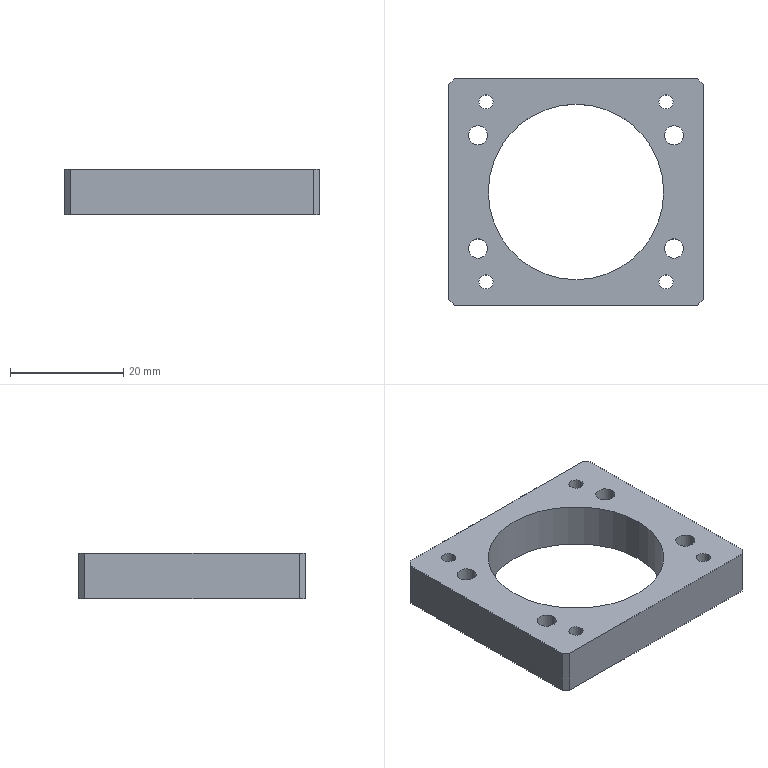Part | NX | features BREP 1 | 1 solid | 40 faces | box 45 x 40 x 8 mm | volume 7532 mm3 | cylinder 26 | plane 14 | commonest cylinder face diameters 2.5 x8 3.4 x8 6.7 x8 31 x2
STEP:
#1=CARTESIAN_POINT('',(-14.66,15.91,8.));
#2=VERTEX_POINT('',#1);
#3=CARTESIAN_POINT('',(-17.16,15.91,8.));
#4=VERTEX_POINT('',#3);
#5=CARTESIAN_POINT('',(-15.91,15.91,8.));
#6=DIRECTION('',(0.,0.,-1.));
#7=DIRECTION('',(-1.,0.,0.));
#8=AXIS2_PLACEMENT_3D('',#5,#6,#7);
#9=CIRCLE('',#8,1.25);
#10=EDGE_CURVE('',#2,#4,#9,.T.);
#11=ORIENTED_EDGE('',*,*,#10,.F.);
#12=CARTESIAN_POINT('',(-14.66,15.91,0.));
#13=VERTEX_POINT('',#12);
#14=CARTESIAN_POINT('',(-14.66,15.91,0.));
#15=DIRECTION('',(0.,0.,-1.));
#16=VECTOR('',#15,1000.);
#17=LINE('',#14,#16);
#18=EDGE_CURVE('',#2,#13,#17,.T.);
#19=ORIENTED_EDGE('',*,*,#18,.T.);
#20=CARTESIAN_POINT('',(-17.16,15.91,0.));
#21=VERTEX_POINT('',#20);
#22=CARTESIAN_POINT('',(-15.91,15.91,0.));
#23=DIRECTION('',(0.,0.,-1.));
#24=DIRECTION('',(-1.,0.,0.));
#25=AXIS2_PLACEMENT_3D('',#22,#23,#24);
#26=CIRCLE('',#25,1.25);
#27=EDGE_CURVE('',#13,#21,#26,.T.);
#28=ORIENTED_EDGE('',*,*,#27,.T.);
#29=CARTESIAN_POINT('',(-17.16,15.91,0.));
#30=DIRECTION('',(0.,0.,-1.));
#31=VECTOR('',#30,1000.);
#32=LINE('',#29,#31);
#33=EDGE_CURVE('',#4,#21,#32,.T.);
#34=ORIENTED_EDGE('',*,*,#33,.F.);
#35=EDGE_LOOP('',(#11,#19,#28,#34));
#36=FACE_BOUND('',#35,.T.);
#37=CARTESIAN_POINT('',(-15.91,15.91,0.));
#38=DIRECTION('',(0.,0.,-1.));
#39=DIRECTION('',(-1.,0.,0.));
#40=AXIS2_PLACEMENT_3D('',#37,#38,#39);
#41=CYLINDRICAL_SURFACE('',#40,1.25);
#42=ADVANCED_FACE('',(#36),#41,.F.);
#43=CARTESIAN_POINT('',(17.16,15.91,8.));
#44=VERTEX_POINT('',#43);
#45=CARTESIAN_POINT('',(14.66,15.91,8.));
#46=VERTEX_POINT('',#45);
#47=CARTESIAN_POINT('',(15.91,15.91,8.));
#48=DIRECTION('',(0.,0.,-1.));
#49=DIRECTION('',(-1.,0.,0.));
#50=AXIS2_PLACEMENT_3D('',#47,#48,#49);
#51=CIRCLE('',#50,1.25);
#52=EDGE_CURVE('',#44,#46,#51,.T.);
#53=ORIENTED_EDGE('',*,*,#52,.F.);
#54=CARTESIAN_POINT('',(17.16,15.91,0.));
#55=VERTEX_POINT('',#54);
#56=CARTESIAN_POINT('',(17.16,15.91,0.));
#57=DIRECTION('',(0.,0.,-1.));
#58=VECTOR('',#57,1000.);
#59=LINE('',#56,#58);
#60=EDGE_CURVE('',#44,#55,#59,.T.);
#61=ORIENTED_EDGE('',*,*,#60,.T.);
#62=CARTESIAN_POINT('',(14.66,15.91,0.));
#63=VERTEX_POINT('',#62);
#64=CARTESIAN_POINT('',(15.91,15.91,0.));
#65=DIRECTION('',(0.,0.,-1.));
#66=DIRECTION('',(-1.,0.,0.));
#67=AXIS2_PLACEMENT_3D('',#64,#65,#66);
#68=CIRCLE('',#67,1.25);
#69=EDGE_CURVE('',#55,#63,#68,.T.);
#70=ORIENTED_EDGE('',*,*,#69,.T.);
#71=CARTESIAN_POINT('',(14.66,15.91,0.));
#72=DIRECTION('',(0.,0.,-1.));
#73=VECTOR('',#72,1000.);
#74=LINE('',#71,#73);
#75=EDGE_CURVE('',#46,#63,#74,.T.);
#76=ORIENTED_EDGE('',*,*,#75,.F.);
#77=EDGE_LOOP('',(#53,#61,#70,#76));
#78=FACE_BOUND('',#77,.T.);
#79=CARTESIAN_POINT('',(15.91,15.91,0.));
#80=DIRECTION('',(0.,0.,-1.));
#81=DIRECTION('',(-1.,0.,0.));
#82=AXIS2_PLACEMENT_3D('',#79,#80,#81);
#83=CYLINDRICAL_SURFACE('',#82,1.25);
#84=ADVANCED_FACE('',(#78),#83,.F.);
#85=CARTESIAN_POINT('',(17.16,-15.91,8.));
#86=VERTEX_POINT('',#85);
#87=CARTESIAN_POINT('',(14.66,-15.91,8.));
#88=VERTEX_POINT('',#87);
#89=CARTESIAN_POINT('',(15.91,-15.91,8.));
#90=DIRECTION('',(0.,0.,-1.));
#91=DIRECTION('',(-1.,0.,0.));
#92=AXIS2_PLACEMENT_3D('',#89,#90,#91);
#93=CIRCLE('',#92,1.25);
#94=EDGE_CURVE('',#86,#88,#93,.T.);
#95=ORIENTED_EDGE('',*,*,#94,.F.);
#96=CARTESIAN_POINT('',(17.16,-15.91,0.));
#97=VERTEX_POINT('',#96);
#98=CARTESIAN_POINT('',(17.16,-15.91,0.));
#99=DIRECTION('',(0.,0.,-1.));
#100=VECTOR('',#99,1000.);
#101=LINE('',#98,#100);
#102=EDGE_CURVE('',#86,#97,#101,.T.);
#103=ORIENTED_EDGE('',*,*,#102,.T.);
#104=CARTESIAN_POINT('',(14.66,-15.91,0.));
#105=VERTEX_POINT('',#104);
#106=CARTESIAN_POINT('',(15.91,-15.91,0.));
#107=DIRECTION('',(0.,0.,-1.));
#108=DIRECTION('',(-1.,0.,0.));
#109=AXIS2_PLACEMENT_3D('',#106,#107,#108);
#110=CIRCLE('',#109,1.25);
#111=EDGE_CURVE('',#97,#105,#110,.T.);
#112=ORIENTED_EDGE('',*,*,#111,.T.);
#113=CARTESIAN_POINT('',(14.66,-15.91,0.));
#114=DIRECTION('',(0.,0.,-1.));
#115=VECTOR('',#114,1000.);
#116=LINE('',#113,#115);
#117=EDGE_CURVE('',#88,#105,#116,.T.);
#118=ORIENTED_EDGE('',*,*,#117,.F.);
#119=EDGE_LOOP('',(#95,#103,#112,#118));
#120=FACE_BOUND('',#119,.T.);
#121=CARTESIAN_POINT('',(15.91,-15.91,0.));
#122=DIRECTION('',(0.,0.,-1.));
#123=DIRECTION('',(-1.,0.,0.));
#124=AXIS2_PLACEMENT_3D('',#121,#122,#123);
#125=CYLINDRICAL_SURFACE('',#124,1.25);
#126=ADVANCED_FACE('',(#120),#125,.F.);
#127=CARTESIAN_POINT('',(-14.66,-15.91,8.));
#128=VERTEX_POINT('',#127);
#129=CARTESIAN_POINT('',(-17.16,-15.91,8.));
#130=VERTEX_POINT('',#129);
#131=CARTESIAN_POINT('',(-15.91,-15.91,8.));
#132=DIRECTION('',(0.,0.,-1.));
#133=DIRECTION('',(-1.,0.,0.));
#134=AXIS2_PLACEMENT_3D('',#131,#132,#133);
#135=CIRCLE('',#134,1.25);
#136=EDGE_CURVE('',#128,#130,#135,.T.);
#137=ORIENTED_EDGE('',*,*,#136,.F.);
#138=CARTESIAN_POINT('',(-14.66,-15.91,0.));
#139=VERTEX_POINT('',#138);
#140=CARTESIAN_POINT('',(-14.66,-15.91,0.));
#141=DIRECTION('',(0.,0.,-1.));
#142=VECTOR('',#141,1000.);
#143=LINE('',#140,#142);
#144=EDGE_CURVE('',#128,#139,#143,.T.);
#145=ORIENTED_EDGE('',*,*,#144,.T.);
#146=CARTESIAN_POINT('',(-17.16,-15.91,0.));
#147=VERTEX_POINT('',#146);
#148=CARTESIAN_POINT('',(-15.91,-15.91,0.));
#149=DIRECTION('',(0.,0.,-1.));
#150=DIRECTION('',(-1.,0.,0.));
#151=AXIS2_PLACEMENT_3D('',#148,#149,#150);
#152=CIRCLE('',#151,1.25);
#153=EDGE_CURVE('',#139,#147,#152,.T.);
#154=ORIENTED_EDGE('',*,*,#153,.T.);
#155=CARTESIAN_POINT('',(-17.16,-15.91,0.));
#156=DIRECTION('',(0.,0.,-1.));
#157=VECTOR('',#156,1000.);
#158=LINE('',#155,#157);
#159=EDGE_CURVE('',#130,#147,#158,.T.);
#160=ORIENTED_EDGE('',*,*,#159,.F.);
#161=EDGE_LOOP('',(#137,#145,#154,#160));
#162=FACE_BOUND('',#161,.T.);
#163=CARTESIAN_POINT('',(-15.91,-15.91,0.));
#164=DIRECTION('',(0.,0.,-1.));
#165=DIRECTION('',(-1.,0.,0.));
#166=AXIS2_PLACEMENT_3D('',#163,#164,#165);
#167=CYLINDRICAL_SURFACE('',#166,1.25);
#168=ADVANCED_FACE('',(#162),#167,.F.);
#169=CARTESIAN_POINT('',(-13.971,-10.,3.5));
#170=VERTEX_POINT('',#169);
#171=CARTESIAN_POINT('',(-20.671,-10.,3.5));
#172=VERTEX_POINT('',#171);
#173=CARTESIAN_POINT('',(-17.321,-10.,3.5));
#174=DIRECTION('',(0.,0.,-1.));
#175=DIRECTION('',(-1.,0.,0.));
#176=AXIS2_PLACEMENT_3D('',#173,#174,#175);
#177=CIRCLE('',#176,3.35);
#178=EDGE_CURVE('',#170,#172,#177,.T.);
#179=ORIENTED_EDGE('',*,*,#178,.F.);
#180=CARTESIAN_POINT('',(-13.971,-10.,0.));
#181=VERTEX_POINT('',#180);
#182=CARTESIAN_POINT('',(-13.971,-10.,0.));
#183=DIRECTION('',(0.,0.,-1.));
#184=VECTOR('',#183,1000.);
#185=LINE('',#182,#184);
#186=EDGE_CURVE('',#170,#181,#185,.T.);
#187=ORIENTED_EDGE('',*,*,#186,.T.);
#188=CARTESIAN_POINT('',(-20.671,-10.,0.));
#189=VERTEX_POINT('',#188);
#190=CARTESIAN_POINT('',(-17.321,-10.,0.));
#191=DIRECTION('',(0.,0.,-1.));
#192=DIRECTION('',(-1.,0.,0.));
#193=AXIS2_PLACEMENT_3D('',#190,#191,#192);
#194=CIRCLE('',#193,3.35);
#195=EDGE_CURVE('',#181,#189,#194,.T.);
#196=ORIENTED_EDGE('',*,*,#195,.T.);
#197=CARTESIAN_POINT('',(-20.671,-10.,0.));
#198=DIRECTION('',(0.,0.,-1.));
#199=VECTOR('',#198,1000.);
#200=LINE('',#197,#199);
#201=EDGE_CURVE('',#172,#189,#200,.T.);
#202=ORIENTED_EDGE('',*,*,#201,.F.);
#203=EDGE_LOOP('',(#179,#187,#196,#202));
#204=FACE_BOUND('',#203,.T.);
#205=CARTESIAN_POINT('',(-17.321,-10.,0.));
#206=DIRECTION('',(0.,0.,-1.));
#207=DIRECTION('',(-1.,0.,0.));
#208=AXIS2_PLACEMENT_3D('',#205,#206,#207);
#209=CYLINDRICAL_SURFACE('',#208,3.35);
#210=ADVANCED_FACE('',(#204),#209,.F.);
#211=CARTESIAN_POINT('',(-15.621,-10.,8.));
#212=VERTEX_POINT('',#211);
#213=CARTESIAN_POINT('',(-19.021,-10.,8.));
#214=VERTEX_POINT('',#213);
#215=CARTESIAN_POINT('',(-17.321,-10.,8.));
#216=DIRECTION('',(0.,0.,-1.));
#217=DIRECTION('',(-1.,0.,0.));
#218=AXIS2_PLACEMENT_3D('',#215,#216,#217);
#219=CIRCLE('',#218,1.7);
#220=EDGE_CURVE('',#212,#214,#219,.T.);
#221=ORIENTED_EDGE('',*,*,#220,.F.);
#222=CARTESIAN_POINT('',(-15.621,-10.,3.5));
#223=VERTEX_POINT('',#222);
#224=CARTESIAN_POINT('',(-15.621,-10.,0.));
#225=DIRECTION('',(0.,0.,-1.));
#226=VECTOR('',#225,1000.);
#227=LINE('',#224,#226);
#228=EDGE_CURVE('',#212,#223,#227,.T.);
#229=ORIENTED_EDGE('',*,*,#228,.T.);
#230=CARTESIAN_POINT('',(-19.021,-10.,3.5));
#231=VERTEX_POINT('',#230);
#232=CARTESIAN_POINT('',(-17.321,-10.,3.5));
#233=DIRECTION('',(0.,0.,-1.));
#234=DIRECTION('',(-1.,0.,0.));
#235=AXIS2_PLACEMENT_3D('',#232,#233,#234);
#236=CIRCLE('',#235,1.7);
#237=EDGE_CURVE('',#223,#231,#236,.T.);
#238=ORIENTED_EDGE('',*,*,#237,.T.);
#239=CARTESIAN_POINT('',(-19.021,-10.,0.));
#240=DIRECTION('',(0.,0.,-1.));
#241=VECTOR('',#240,1000.);
#242=LINE('',#239,#241);
#243=EDGE_CURVE('',#214,#231,#242,.T.);
#244=ORIENTED_EDGE('',*,*,#243,.F.);
#245=EDGE_LOOP('',(#221,#229,#238,#244));
#246=FACE_BOUND('',#245,.T.);
#247=CARTESIAN_POINT('',(-17.321,-10.,0.));
#248=DIRECTION('',(0.,0.,-1.));
#249=DIRECTION('',(-1.,0.,0.));
#250=AXIS2_PLACEMENT_3D('',#247,#248,#249);
#251=CYLINDRICAL_SURFACE('',#250,1.7);
#252=ADVANCED_FACE('',(#246),#251,.F.);
#253=CARTESIAN_POINT('',(-13.971,10.,3.5));
#254=VERTEX_POINT('',#253);
#255=CARTESIAN_POINT('',(-20.671,10.,3.5));
#256=VERTEX_POINT('',#255);
#257=CARTESIAN_POINT('',(-17.321,10.,3.5));
#258=DIRECTION('',(0.,0.,-1.));
#259=DIRECTION('',(-1.,0.,0.));
#260=AXIS2_PLACEMENT_3D('',#257,#258,#259);
#261=CIRCLE('',#260,3.35);
#262=EDGE_CURVE('',#254,#256,#261,.T.);
#263=ORIENTED_EDGE('',*,*,#262,.F.);
#264=CARTESIAN_POINT('',(-13.971,10.,0.));
#265=VERTEX_POINT('',#264);
#266=CARTESIAN_POINT('',(-13.971,10.,0.));
#267=DIRECTION('',(0.,0.,-1.));
#268=VECTOR('',#267,1000.);
#269=LINE('',#266,#268);
#270=EDGE_CURVE('',#254,#265,#269,.T.);
#271=ORIENTED_EDGE('',*,*,#270,.T.);
#272=CARTESIAN_POINT('',(-20.671,10.,0.));
#273=VERTEX_POINT('',#272);
#274=CARTESIAN_POINT('',(-17.321,10.,0.));
#275=DIRECTION('',(0.,0.,-1.));
#276=DIRECTION('',(-1.,0.,0.));
#277=AXIS2_PLACEMENT_3D('',#274,#275,#276);
#278=CIRCLE('',#277,3.35);
#279=EDGE_CURVE('',#265,#273,#278,.T.);
#280=ORIENTED_EDGE('',*,*,#279,.T.);
#281=CARTESIAN_POINT('',(-20.671,10.,0.));
#282=DIRECTION('',(0.,0.,-1.));
#283=VECTOR('',#282,1000.);
#284=LINE('',#281,#283);
#285=EDGE_CURVE('',#256,#273,#284,.T.);
#286=ORIENTED_EDGE('',*,*,#285,.F.);
#287=EDGE_LOOP('',(#263,#271,#280,#286));
#288=FACE_BOUND('',#287,.T.);
#289=CARTESIAN_POINT('',(-17.321,10.,0.));
#290=DIRECTION('',(0.,0.,-1.));
#291=DIRECTION('',(-1.,0.,0.));
#292=AXIS2_PLACEMENT_3D('',#289,#290,#291);
#293=CYLINDRICAL_SURFACE('',#292,3.35);
#294=ADVANCED_FACE('',(#288),#293,.F.);
#295=CARTESIAN_POINT('',(-15.621,10.,8.));
#296=VERTEX_POINT('',#295);
#297=CARTESIAN_POINT('',(-19.021,10.,8.));
#298=VERTEX_POINT('',#297);
#299=CARTESIAN_POINT('',(-17.321,10.,8.));
#300=DIRECTION('',(0.,0.,-1.));
#301=DIRECTION('',(-1.,0.,0.));
#302=AXIS2_PLACEMENT_3D('',#299,#300,#301);
#303=CIRCLE('',#302,1.7);
#304=EDGE_CURVE('',#296,#298,#303,.T.);
#305=ORIENTED_EDGE('',*,*,#304,.F.);
#306=CARTESIAN_POINT('',(-15.621,10.,3.5));
#307=VERTEX_POINT('',#306);
#308=CARTESIAN_POINT('',(-15.621,10.,0.));
#309=DIRECTION('',(0.,0.,-1.));
#310=VECTOR('',#309,1000.);
#311=LINE('',#308,#310);
#312=EDGE_CURVE('',#296,#307,#311,.T.);
#313=ORIENTED_EDGE('',*,*,#312,.T.);
#314=CARTESIAN_POINT('',(-19.021,10.,3.5));
#315=VERTEX_POINT('',#314);
#316=CARTESIAN_POINT('',(-17.321,10.,3.5));
#317=DIRECTION('',(0.,0.,-1.));
#318=DIRECTION('',(-1.,0.,0.));
#319=AXIS2_PLACEMENT_3D('',#316,#317,#318);
#320=CIRCLE('',#319,1.7);
#321=EDGE_CURVE('',#307,#315,#320,.T.);
#322=ORIENTED_EDGE('',*,*,#321,.T.);
#323=CARTESIAN_POINT('',(-19.021,10.,0.));
#324=DIRECTION('',(0.,0.,-1.));
#325=VECTOR('',#324,1000.);
#326=LINE('',#323,#325);
#327=EDGE_CURVE('',#298,#315,#326,.T.);
#328=ORIENTED_EDGE('',*,*,#327,.F.);
#329=EDGE_LOOP('',(#305,#313,#322,#328));
#330=FACE_BOUND('',#329,.T.);
#331=CARTESIAN_POINT('',(-17.321,10.,0.));
#332=DIRECTION('',(0.,0.,-1.));
#333=DIRECTION('',(-1.,0.,0.));
#334=AXIS2_PLACEMENT_3D('',#331,#332,#333);
#335=CYLINDRICAL_SURFACE('',#334,1.7);
#336=ADVANCED_FACE('',(#330),#335,.F.);
#337=CARTESIAN_POINT('',(20.671,10.,3.5));
#338=VERTEX_POINT('',#337);
#339=CARTESIAN_POINT('',(13.971,10.,3.5));
#340=VERTEX_POINT('',#339);
#341=CARTESIAN_POINT('',(17.321,10.,3.5));
#342=DIRECTION('',(0.,0.,-1.));
#343=DIRECTION('',(-1.,0.,0.));
#344=AXIS2_PLACEMENT_3D('',#341,#342,#343);
#345=CIRCLE('',#344,3.35);
#346=EDGE_CURVE('',#338,#340,#345,.T.);
#347=ORIENTED_EDGE('',*,*,#346,.F.);
#348=CARTESIAN_POINT('',(20.671,10.,0.));
#349=VERTEX_POINT('',#348);
#350=CARTESIAN_POINT('',(20.671,10.,0.));
#351=DIRECTION('',(0.,0.,-1.));
#352=VECTOR('',#351,1000.);
#353=LINE('',#350,#352);
#354=EDGE_CURVE('',#338,#349,#353,.T.);
#355=ORIENTED_EDGE('',*,*,#354,.T.);
#356=CARTESIAN_POINT('',(13.971,10.,0.));
#357=VERTEX_POINT('',#356);
#358=CARTESIAN_POINT('',(17.321,10.,0.));
#359=DIRECTION('',(0.,0.,-1.));
#360=DIRECTION('',(-1.,0.,0.));
#361=AXIS2_PLACEMENT_3D('',#358,#359,#360);
#362=CIRCLE('',#361,3.35);
#363=EDGE_CURVE('',#349,#357,#362,.T.);
#364=ORIENTED_EDGE('',*,*,#363,.T.);
#365=CARTESIAN_POINT('',(13.971,10.,0.));
#366=DIRECTION('',(0.,0.,-1.));
#367=VECTOR('',#366,1000.);
#368=LINE('',#365,#367);
#369=EDGE_CURVE('',#340,#357,#368,.T.);
#370=ORIENTED_EDGE('',*,*,#369,.F.);
#371=EDGE_LOOP('',(#347,#355,#364,#370));
#372=FACE_BOUND('',#371,.T.);
#373=CARTESIAN_POINT('',(17.321,10.,0.));
#374=DIRECTION('',(0.,0.,-1.));
#375=DIRECTION('',(-1.,0.,0.));
#376=AXIS2_PLACEMENT_3D('',#373,#374,#375);
#377=CYLINDRICAL_SURFACE('',#376,3.35);
#378=ADVANCED_FACE('',(#372),#377,.F.);
#379=CARTESIAN_POINT('',(19.021,10.,8.));
#380=VERTEX_POINT('',#379);
#381=CARTESIAN_POINT('',(15.621,10.,8.));
#382=VERTEX_POINT('',#381);
#383=CARTESIAN_POINT('',(17.321,10.,8.));
#384=DIRECTION('',(0.,0.,-1.));
#385=DIRECTION('',(-1.,0.,0.));
#386=AXIS2_PLACEMENT_3D('',#383,#384,#385);
#387=CIRCLE('',#386,1.7);
#388=EDGE_CURVE('',#380,#382,#387,.T.);
#389=ORIENTED_EDGE('',*,*,#388,.F.);
#390=CARTESIAN_POINT('',(19.021,10.,3.5));
#391=VERTEX_POINT('',#390);
#392=CARTESIAN_POINT('',(19.021,10.,0.));
#393=DIRECTION('',(0.,0.,-1.));
#394=VECTOR('',#393,1000.);
#395=LINE('',#392,#394);
#396=EDGE_CURVE('',#380,#391,#395,.T.);
#397=ORIENTED_EDGE('',*,*,#396,.T.);
#398=CARTESIAN_POINT('',(15.621,10.,3.5));
#399=VERTEX_POINT('',#398);
#400=CARTESIAN_POINT('',(17.321,10.,3.5));
#401=DIRECTION('',(0.,0.,-1.));
#402=DIRECTION('',(-1.,0.,0.));
#403=AXIS2_PLACEMENT_3D('',#400,#401,#402);
#404=CIRCLE('',#403,1.7);
#405=EDGE_CURVE('',#391,#399,#404,.T.);
#406=ORIENTED_EDGE('',*,*,#405,.T.);
#407=CARTESIAN_POINT('',(15.621,10.,0.));
#408=DIRECTION('',(0.,0.,-1.));
#409=VECTOR('',#408,1000.);
#410=LINE('',#407,#409);
#411=EDGE_CURVE('',#382,#399,#410,.T.);
#412=ORIENTED_EDGE('',*,*,#411,.F.);
#413=EDGE_LOOP('',(#389,#397,#406,#412));
#414=FACE_BOUND('',#413,.T.);
#415=CARTESIAN_POINT('',(17.321,10.,0.));
#416=DIRECTION('',(0.,0.,-1.));
#417=DIRECTION('',(-1.,0.,0.));
#418=AXIS2_PLACEMENT_3D('',#415,#416,#417);
#419=CYLINDRICAL_SURFACE('',#418,1.7);
#420=ADVANCED_FACE('',(#414),#419,.F.);
#421=CARTESIAN_POINT('',(20.671,-10.,3.5));
#422=VERTEX_POINT('',#421);
#423=CARTESIAN_POINT('',(13.971,-10.,3.5));
#424=VERTEX_POINT('',#423);
#425=CARTESIAN_POINT('',(17.321,-10.,3.5));
#426=DIRECTION('',(0.,0.,-1.));
#427=DIRECTION('',(-1.,0.,0.));
#428=AXIS2_PLACEMENT_3D('',#425,#426,#427);
#429=CIRCLE('',#428,3.35);
#430=EDGE_CURVE('',#422,#424,#429,.T.);
#431=ORIENTED_EDGE('',*,*,#430,.F.);
#432=CARTESIAN_POINT('',(20.671,-10.,0.));
#433=VERTEX_POINT('',#432);
#434=CARTESIAN_POINT('',(20.671,-10.,0.));
#435=DIRECTION('',(0.,0.,-1.));
#436=VECTOR('',#435,1000.);
#437=LINE('',#434,#436);
#438=EDGE_CURVE('',#422,#433,#437,.T.);
#439=ORIENTED_EDGE('',*,*,#438,.T.);
#440=CARTESIAN_POINT('',(13.971,-10.,0.));
#441=VERTEX_POINT('',#440);
#442=CARTESIAN_POINT('',(17.321,-10.,0.));
#443=DIRECTION('',(0.,0.,-1.));
#444=DIRECTION('',(-1.,0.,0.));
#445=AXIS2_PLACEMENT_3D('',#442,#443,#444);
#446=CIRCLE('',#445,3.35);
#447=EDGE_CURVE('',#433,#441,#446,.T.);
#448=ORIENTED_EDGE('',*,*,#447,.T.);
#449=CARTESIAN_POINT('',(13.971,-10.,0.));
#450=DIRECTION('',(0.,0.,-1.));
#451=VECTOR('',#450,1000.);
#452=LINE('',#449,#451);
#453=EDGE_CURVE('',#424,#441,#452,.T.);
#454=ORIENTED_EDGE('',*,*,#453,.F.);
#455=EDGE_LOOP('',(#431,#439,#448,#454));
#456=FACE_BOUND('',#455,.T.);
#457=CARTESIAN_POINT('',(17.321,-10.,0.));
#458=DIRECTION('',(0.,0.,-1.));
#459=DIRECTION('',(-1.,0.,0.));
#460=AXIS2_PLACEMENT_3D('',#457,#458,#459);
#461=CYLINDRICAL_SURFACE('',#460,3.35);
#462=ADVANCED_FACE('',(#456),#461,.F.);
#463=CARTESIAN_POINT('',(19.021,-10.,8.));
#464=VERTEX_POINT('',#463);
#465=CARTESIAN_POINT('',(15.621,-10.,8.));
#466=VERTEX_POINT('',#465);
#467=CARTESIAN_POINT('',(17.321,-10.,8.));
#468=DIRECTION('',(0.,0.,-1.));
#469=DIRECTION('',(-1.,0.,0.));
#470=AXIS2_PLACEMENT_3D('',#467,#468,#469);
#471=CIRCLE('',#470,1.7);
#472=EDGE_CURVE('',#464,#466,#471,.T.);
#473=ORIENTED_EDGE('',*,*,#472,.F.);
#474=CARTESIAN_POINT('',(19.021,-10.,3.5));
#475=VERTEX_POINT('',#474);
#476=CARTESIAN_POINT('',(19.021,-10.,0.));
#477=DIRECTION('',(0.,0.,-1.));
#478=VECTOR('',#477,1000.);
#479=LINE('',#476,#478);
#480=EDGE_CURVE('',#464,#475,#479,.T.);
#481=ORIENTED_EDGE('',*,*,#480,.T.);
#482=CARTESIAN_POINT('',(15.621,-10.,3.5));
#483=VERTEX_POINT('',#482);
#484=CARTESIAN_POINT('',(17.321,-10.,3.5));
#485=DIRECTION('',(0.,0.,-1.));
#486=DIRECTION('',(-1.,0.,0.));
#487=AXIS2_PLACEMENT_3D('',#484,#485,#486);
#488=CIRCLE('',#487,1.7);
#489=EDGE_CURVE('',#475,#483,#488,.T.);
#490=ORIENTED_EDGE('',*,*,#489,.T.);
#491=CARTESIAN_POINT('',(15.621,-10.,0.));
#492=DIRECTION('',(0.,0.,-1.));
#493=VECTOR('',#492,1000.);
#494=LINE('',#491,#493);
#495=EDGE_CURVE('',#466,#483,#494,.T.);
#496=ORIENTED_EDGE('',*,*,#495,.F.);
#497=EDGE_LOOP('',(#473,#481,#490,#496));
#498=FACE_BOUND('',#497,.T.);
#499=CARTESIAN_POINT('',(17.321,-10.,0.));
#500=DIRECTION('',(0.,0.,-1.));
#501=DIRECTION('',(-1.,0.,0.));
#502=AXIS2_PLACEMENT_3D('',#499,#500,#501);
#503=CYLINDRICAL_SURFACE('',#502,1.7);
#504=ADVANCED_FACE('',(#498),#503,.F.);
#505=CARTESIAN_POINT('',(-15.5,0.,0.));
#506=VERTEX_POINT('',#505);
#507=CARTESIAN_POINT('',(15.5,0.,0.));
#508=VERTEX_POINT('',#507);
#509=CARTESIAN_POINT('',(0.,0.,0.));
#510=DIRECTION('',(0.,0.,1.));
#511=DIRECTION('',(1.,0.,0.));
#512=AXIS2_PLACEMENT_3D('',#509,#510,#511);
#513=CIRCLE('',#512,15.5);
#514=EDGE_CURVE('',#506,#508,#513,.T.);
#515=ORIENTED_EDGE('',*,*,#514,.F.);
#516=CARTESIAN_POINT('',(-15.5,0.,8.));
#517=VERTEX_POINT('',#516);
#518=CARTESIAN_POINT('',(-15.5,0.,-20.));
#519=DIRECTION('',(0.,0.,1.));
#520=VECTOR('',#519,1000.);
#521=LINE('',#518,#520);
#522=EDGE_CURVE('',#517,#506,#521,.F.);
#523=ORIENTED_EDGE('',*,*,#522,.F.);
#524=CARTESIAN_POINT('',(15.5,0.,8.));
#525=VERTEX_POINT('',#524);
#526=CARTESIAN_POINT('',(0.,0.,8.));
#527=DIRECTION('',(0.,0.,1.));
#528=DIRECTION('',(1.,0.,0.));
#529=AXIS2_PLACEMENT_3D('',#526,#527,#528);
#530=CIRCLE('',#529,15.5);
#531=EDGE_CURVE('',#517,#525,#530,.T.);
#532=ORIENTED_EDGE('',*,*,#531,.T.);
#533=CARTESIAN_POINT('',(15.5,0.,-20.));
#534=DIRECTION('',(0.,0.,1.));
#535=VECTOR('',#534,1000.);
#536=LINE('',#533,#535);
#537=EDGE_CURVE('',#525,#508,#536,.F.);
#538=ORIENTED_EDGE('',*,*,#537,.T.);
#539=EDGE_LOOP('',(#515,#523,#532,#538));
#540=FACE_BOUND('',#539,.T.);
#541=CARTESIAN_POINT('',(0.,0.,-20.));
#542=DIRECTION('',(0.,0.,1.));
#543=DIRECTION('',(1.,0.,0.));
#544=AXIS2_PLACEMENT_3D('',#541,#542,#543);
#545=CYLINDRICAL_SURFACE('',#544,15.5);
#546=ADVANCED_FACE('',(#540),#545,.F.);
#547=CARTESIAN_POINT('',(22.5,-19.,8.));
#548=VERTEX_POINT('',#547);
#549=CARTESIAN_POINT('',(22.5,19.,8.));
#550=VERTEX_POINT('',#549);
#551=CARTESIAN_POINT('',(22.5,20.,8.));
#552=DIRECTION('',(0.,1.,0.));
#553=VECTOR('',#552,1000.);
#554=LINE('',#551,#553);
#555=EDGE_CURVE('',#548,#550,#554,.T.);
#556=ORIENTED_EDGE('',*,*,#555,.F.);
#557=CARTESIAN_POINT('',(22.5,-19.,0.));
#558=VERTEX_POINT('',#557);
#559=CARTESIAN_POINT('',(22.5,-19.,8.));
#560=DIRECTION('',(0.,0.,-1.));
#561=VECTOR('',#560,1000.);
#562=LINE('',#559,#561);
#563=EDGE_CURVE('',#548,#558,#562,.T.);
#564=ORIENTED_EDGE('',*,*,#563,.T.);
#565=CARTESIAN_POINT('',(22.5,19.,0.));
#566=VERTEX_POINT('',#565);
#567=CARTESIAN_POINT('',(22.5,20.,0.));
#568=DIRECTION('',(0.,1.,0.));
#569=VECTOR('',#568,1000.);
#570=LINE('',#567,#569);
#571=EDGE_CURVE('',#558,#566,#570,.T.);
#572=ORIENTED_EDGE('',*,*,#571,.T.);
#573=CARTESIAN_POINT('',(22.5,19.,8.));
#574=DIRECTION('',(0.,0.,1.));
#575=VECTOR('',#574,1000.);
#576=LINE('',#573,#575);
#577=EDGE_CURVE('',#566,#550,#576,.T.);
#578=ORIENTED_EDGE('',*,*,#577,.T.);
#579=EDGE_LOOP('',(#556,#564,#572,#578));
#580=FACE_BOUND('',#579,.T.);
#581=CARTESIAN_POINT('',(22.5,20.,8.));
#582=DIRECTION('',(-1.,0.,0.));
#583=DIRECTION('',(0.,1.,0.));
#584=AXIS2_PLACEMENT_3D('',#581,#582,#583);
#585=PLANE('',#584);
#586=ADVANCED_FACE('',(#580),#585,.F.);
#587=CARTESIAN_POINT('',(21.5,20.,8.));
#588=VERTEX_POINT('',#587);
#589=CARTESIAN_POINT('',(-21.5,20.,8.));
#590=VERTEX_POINT('',#589);
#591=CARTESIAN_POINT('',(-22.5,20.,8.));
#592=DIRECTION('',(-1.,0.,0.));
#593=VECTOR('',#592,1000.);
#594=LINE('',#591,#593);
#595=EDGE_CURVE('',#588,#590,#594,.T.);
#596=ORIENTED_EDGE('',*,*,#595,.F.);
#597=CARTESIAN_POINT('',(21.5,20.,0.));
#598=VERTEX_POINT('',#597);
#599=CARTESIAN_POINT('',(21.5,20.,8.));
#600=DIRECTION('',(0.,0.,-1.));
#601=VECTOR('',#600,1000.);
#602=LINE('',#599,#601);
#603=EDGE_CURVE('',#588,#598,#602,.T.);
#604=ORIENTED_EDGE('',*,*,#603,.T.);
#605=CARTESIAN_POINT('',(-21.5,20.,0.));
#606=VERTEX_POINT('',#605);
#607=CARTESIAN_POINT('',(-22.5,20.,0.));
#608=DIRECTION('',(-1.,0.,0.));
#609=VECTOR('',#608,1000.);
#610=LINE('',#607,#609);
#611=EDGE_CURVE('',#598,#606,#610,.T.);
#612=ORIENTED_EDGE('',*,*,#611,.T.);
#613=CARTESIAN_POINT('',(-21.5,20.,8.));
#614=DIRECTION('',(0.,0.,1.));
#615=VECTOR('',#614,1000.);
#616=LINE('',#613,#615);
#617=EDGE_CURVE('',#606,#590,#616,.T.);
#618=ORIENTED_EDGE('',*,*,#617,.T.);
#619=EDGE_LOOP('',(#596,#604,#612,#618));
#620=FACE_BOUND('',#619,.T.);
#621=CARTESIAN_POINT('',(-22.5,20.,8.));
#622=DIRECTION('',(0.,-1.,0.));
#623=DIRECTION('',(0.,0.,-1.));
#624=AXIS2_PLACEMENT_3D('',#621,#622,#623);
#625=PLANE('',#624);
#626=ADVANCED_FACE('',(#620),#625,.F.);
#627=CARTESIAN_POINT('',(-22.5,19.,0.));
#628=VERTEX_POINT('',#627);
#629=CARTESIAN_POINT('',(-22.5,-19.,0.));
#630=VERTEX_POINT('',#629);
#631=CARTESIAN_POINT('',(-22.5,20.,0.));
#632=DIRECTION('',(0.,-1.,0.));
#633=VECTOR('',#632,1000.);
#634=LINE('',#631,#633);
#635=EDGE_CURVE('',#628,#630,#634,.T.);
#636=ORIENTED_EDGE('',*,*,#635,.T.);
#637=CARTESIAN_POINT('',(-22.5,-19.,8.));
#638=VERTEX_POINT('',#637);
#639=CARTESIAN_POINT('',(-22.5,-19.,8.));
#640=DIRECTION('',(0.,0.,1.));
#641=VECTOR('',#640,1000.);
#642=LINE('',#639,#641);
#643=EDGE_CURVE('',#630,#638,#642,.T.);
#644=ORIENTED_EDGE('',*,*,#643,.T.);
#645=CARTESIAN_POINT('',(-22.5,19.,8.));
#646=VERTEX_POINT('',#645);
#647=CARTESIAN_POINT('',(-22.5,20.,8.));
#648=DIRECTION('',(0.,-1.,0.));
#649=VECTOR('',#648,1000.);
#650=LINE('',#647,#649);
#651=EDGE_CURVE('',#646,#638,#650,.T.);
#652=ORIENTED_EDGE('',*,*,#651,.F.);
#653=CARTESIAN_POINT('',(-22.5,19.,8.));
#654=DIRECTION('',(0.,0.,-1.));
#655=VECTOR('',#654,1000.);
#656=LINE('',#653,#655);
#657=EDGE_CURVE('',#646,#628,#656,.T.);
#658=ORIENTED_EDGE('',*,*,#657,.T.);
#659=EDGE_LOOP('',(#636,#644,#652,#658));
#660=FACE_BOUND('',#659,.T.);
#661=CARTESIAN_POINT('',(-22.5,20.,8.));
#662=DIRECTION('',(1.,0.,0.));
#663=DIRECTION('',(0.,1.,0.));
#664=AXIS2_PLACEMENT_3D('',#661,#662,#663);
#665=PLANE('',#664);
#666=ADVANCED_FACE('',(#660),#665,.F.);
#667=CARTESIAN_POINT('',(-21.5,-20.,8.));
#668=VERTEX_POINT('',#667);
#669=CARTESIAN_POINT('',(21.5,-20.,8.));
#670=VERTEX_POINT('',#669);
#671=CARTESIAN_POINT('',(-22.5,-20.,8.));
#672=DIRECTION('',(1.,0.,0.));
#673=VECTOR('',#672,1000.);
#674=LINE('',#671,#673);
#675=EDGE_CURVE('',#668,#670,#674,.T.);
#676=ORIENTED_EDGE('',*,*,#675,.F.);
#677=CARTESIAN_POINT('',(-21.5,-20.,0.));
#678=VERTEX_POINT('',#677);
#679=CARTESIAN_POINT('',(-21.5,-20.,8.));
#680=DIRECTION('',(0.,0.,-1.));
#681=VECTOR('',#680,1000.);
#682=LINE('',#679,#681);
#683=EDGE_CURVE('',#668,#678,#682,.T.);
#684=ORIENTED_EDGE('',*,*,#683,.T.);
#685=CARTESIAN_POINT('',(21.5,-20.,0.));
#686=VERTEX_POINT('',#685);
#687=CARTESIAN_POINT('',(-22.5,-20.,0.));
#688=DIRECTION('',(1.,0.,0.));
#689=VECTOR('',#688,1000.);
#690=LINE('',#687,#689);
#691=EDGE_CURVE('',#678,#686,#690,.T.);
#692=ORIENTED_EDGE('',*,*,#691,.T.);
#693=CARTESIAN_POINT('',(21.5,-20.,8.));
#694=DIRECTION('',(0.,0.,1.));
#695=VECTOR('',#694,1000.);
#696=LINE('',#693,#695);
#697=EDGE_CURVE('',#686,#670,#696,.T.);
#698=ORIENTED_EDGE('',*,*,#697,.T.);
#699=EDGE_LOOP('',(#676,#684,#692,#698));
#700=FACE_BOUND('',#699,.T.);
#701=CARTESIAN_POINT('',(-22.5,-20.,8.));
#702=DIRECTION('',(0.,1.,0.));
#703=DIRECTION('',(1.,0.,0.));
#704=AXIS2_PLACEMENT_3D('',#701,#702,#703);
#705=PLANE('',#704);
#706=ADVANCED_FACE('',(#700),#705,.F.);
#707=ORIENTED_EDGE('',*,*,#651,.T.);
#708=CARTESIAN_POINT('',(-20.75,-20.75,8.));
#709=DIRECTION('',(0.7071,-0.7071,0.));
#710=VECTOR('',#709,1000.);
#711=LINE('',#708,#710);
#712=EDGE_CURVE('',#638,#668,#711,.T.);
#713=ORIENTED_EDGE('',*,*,#712,.T.);
#714=ORIENTED_EDGE('',*,*,#675,.T.);
#715=CARTESIAN_POINT('',(20.75,-20.75,8.));
#716=DIRECTION('',(0.7071,0.7071,0.));
#717=VECTOR('',#716,1000.);
#718=LINE('',#715,#717);
#719=EDGE_CURVE('',#670,#548,#718,.T.);
#720=ORIENTED_EDGE('',*,*,#719,.T.);
#721=ORIENTED_EDGE('',*,*,#555,.T.);
#722=CARTESIAN_POINT('',(20.75,20.75,8.));
#723=DIRECTION('',(-0.7071,0.7071,0.));
#724=VECTOR('',#723,1000.);
#725=LINE('',#722,#724);
#726=EDGE_CURVE('',#550,#588,#725,.T.);
#727=ORIENTED_EDGE('',*,*,#726,.T.);
#728=ORIENTED_EDGE('',*,*,#595,.T.);
#729=CARTESIAN_POINT('',(-20.75,20.75,8.));
#730=DIRECTION('',(-0.7071,-0.7071,0.));
#731=VECTOR('',#730,1000.);
#732=LINE('',#729,#731);
#733=EDGE_CURVE('',#590,#646,#732,.T.);
#734=ORIENTED_EDGE('',*,*,#733,.T.);
#735=EDGE_LOOP('',(#707,#713,#714,#720,#721,#727,#728,#734));
#736=FACE_BOUND('',#735,.T.);
#737=CARTESIAN_POINT('',(-15.91,15.91,8.));
#738=DIRECTION('',(0.,0.,-1.));
#739=DIRECTION('',(-1.,0.,0.));
#740=AXIS2_PLACEMENT_3D('',#737,#738,#739);
#741=CIRCLE('',#740,1.25);
#742=EDGE_CURVE('',#4,#2,#741,.T.);
#743=ORIENTED_EDGE('',*,*,#742,.T.);
#744=ORIENTED_EDGE('',*,*,#10,.T.);
#745=EDGE_LOOP('',(#743,#744));
#746=FACE_BOUND('',#745,.T.);
#747=CARTESIAN_POINT('',(15.91,15.91,8.));
#748=DIRECTION('',(0.,0.,-1.));
#749=DIRECTION('',(-1.,0.,0.));
#750=AXIS2_PLACEMENT_3D('',#747,#748,#749);
#751=CIRCLE('',#750,1.25);
#752=EDGE_CURVE('',#46,#44,#751,.T.);
#753=ORIENTED_EDGE('',*,*,#752,.T.);
#754=ORIENTED_EDGE('',*,*,#52,.T.);
#755=EDGE_LOOP('',(#753,#754));
#756=FACE_BOUND('',#755,.T.);
#757=CARTESIAN_POINT('',(15.91,-15.91,8.));
#758=DIRECTION('',(0.,0.,-1.));
#759=DIRECTION('',(-1.,0.,0.));
#760=AXIS2_PLACEMENT_3D('',#757,#758,#759);
#761=CIRCLE('',#760,1.25);
#762=EDGE_CURVE('',#88,#86,#761,.T.);
#763=ORIENTED_EDGE('',*,*,#762,.T.);
#764=ORIENTED_EDGE('',*,*,#94,.T.);
#765=EDGE_LOOP('',(#763,#764));
#766=FACE_BOUND('',#765,.T.);
#767=CARTESIAN_POINT('',(-15.91,-15.91,8.));
#768=DIRECTION('',(0.,0.,-1.));
#769=DIRECTION('',(-1.,0.,0.));
#770=AXIS2_PLACEMENT_3D('',#767,#768,#769);
#771=CIRCLE('',#770,1.25);
#772=EDGE_CURVE('',#130,#128,#771,.T.);
#773=ORIENTED_EDGE('',*,*,#772,.T.);
#774=ORIENTED_EDGE('',*,*,#136,.T.);
#775=EDGE_LOOP('',(#773,#774));
#776=FACE_BOUND('',#775,.T.);
#777=CARTESIAN_POINT('',(-17.321,-10.,8.));
#778=DIRECTION('',(0.,0.,-1.));
#779=DIRECTION('',(-1.,0.,0.));
#780=AXIS2_PLACEMENT_3D('',#777,#778,#779);
#781=CIRCLE('',#780,1.7);
#782=EDGE_CURVE('',#214,#212,#781,.T.);
#783=ORIENTED_EDGE('',*,*,#782,.T.);
#784=ORIENTED_EDGE('',*,*,#220,.T.);
#785=EDGE_LOOP('',(#783,#784));
#786=FACE_BOUND('',#785,.T.);
#787=CARTESIAN_POINT('',(-17.321,10.,8.));
#788=DIRECTION('',(0.,0.,-1.));
#789=DIRECTION('',(-1.,0.,0.));
#790=AXIS2_PLACEMENT_3D('',#787,#788,#789);
#791=CIRCLE('',#790,1.7);
#792=EDGE_CURVE('',#298,#296,#791,.T.);
#793=ORIENTED_EDGE('',*,*,#792,.T.);
#794=ORIENTED_EDGE('',*,*,#304,.T.);
#795=EDGE_LOOP('',(#793,#794));
#796=FACE_BOUND('',#795,.T.);
#797=CARTESIAN_POINT('',(17.321,10.,8.));
#798=DIRECTION('',(0.,0.,-1.));
#799=DIRECTION('',(-1.,0.,0.));
#800=AXIS2_PLACEMENT_3D('',#797,#798,#799);
#801=CIRCLE('',#800,1.7);
#802=EDGE_CURVE('',#382,#380,#801,.T.);
#803=ORIENTED_EDGE('',*,*,#802,.T.);
#804=ORIENTED_EDGE('',*,*,#388,.T.);
#805=EDGE_LOOP('',(#803,#804));
#806=FACE_BOUND('',#805,.T.);
#807=CARTESIAN_POINT('',(17.321,-10.,8.));
#808=DIRECTION('',(0.,0.,-1.));
#809=DIRECTION('',(-1.,0.,0.));
#810=AXIS2_PLACEMENT_3D('',#807,#808,#809);
#811=CIRCLE('',#810,1.7);
#812=EDGE_CURVE('',#466,#464,#811,.T.);
#813=ORIENTED_EDGE('',*,*,#812,.T.);
#814=ORIENTED_EDGE('',*,*,#472,.T.);
#815=EDGE_LOOP('',(#813,#814));
#816=FACE_BOUND('',#815,.T.);
#817=CARTESIAN_POINT('',(0.,0.,8.));
#818=DIRECTION('',(0.,0.,1.));
#819=DIRECTION('',(1.,0.,0.));
#820=AXIS2_PLACEMENT_3D('',#817,#818,#819);
#821=CIRCLE('',#820,15.5);
#822=EDGE_CURVE('',#525,#517,#821,.T.);
#823=ORIENTED_EDGE('',*,*,#822,.F.);
#824=ORIENTED_EDGE('',*,*,#531,.F.);
#825=EDGE_LOOP('',(#823,#824));
#826=FACE_BOUND('',#825,.T.);
#827=CARTESIAN_POINT('',(0.,0.,8.));
#828=DIRECTION('',(0.,0.,1.));
#829=DIRECTION('',(1.,0.,0.));
#830=AXIS2_PLACEMENT_3D('',#827,#828,#829);
#831=PLANE('',#830);
#832=ADVANCED_FACE('',(#736,#746,#756,#766,#776,#786,#796,#806,#816,#826),#831,.T.);
#833=ORIENTED_EDGE('',*,*,#691,.F.);
#834=CARTESIAN_POINT('',(-21.5,-20.,0.));
#835=DIRECTION('',(-0.7071,0.7071,0.));
#836=VECTOR('',#835,1000.);
#837=LINE('',#834,#836);
#838=EDGE_CURVE('',#678,#630,#837,.T.);
#839=ORIENTED_EDGE('',*,*,#838,.T.);
#840=ORIENTED_EDGE('',*,*,#635,.F.);
#841=CARTESIAN_POINT('',(-22.5,19.,0.));
#842=DIRECTION('',(0.7071,0.7071,0.));
#843=VECTOR('',#842,1000.);
#844=LINE('',#841,#843);
#845=EDGE_CURVE('',#628,#606,#844,.T.);
#846=ORIENTED_EDGE('',*,*,#845,.T.);
#847=ORIENTED_EDGE('',*,*,#611,.F.);
#848=CARTESIAN_POINT('',(21.5,20.,0.));
#849=DIRECTION('',(0.7071,-0.7071,0.));
#850=VECTOR('',#849,1000.);
#851=LINE('',#848,#850);
#852=EDGE_CURVE('',#598,#566,#851,.T.);
#853=ORIENTED_EDGE('',*,*,#852,.T.);
#854=ORIENTED_EDGE('',*,*,#571,.F.);
#855=CARTESIAN_POINT('',(22.5,-19.,0.));
#856=DIRECTION('',(-0.7071,-0.7071,0.));
#857=VECTOR('',#856,1000.);
#858=LINE('',#855,#857);
#859=EDGE_CURVE('',#558,#686,#858,.T.);
#860=ORIENTED_EDGE('',*,*,#859,.T.);
#861=EDGE_LOOP('',(#833,#839,#840,#846,#847,#853,#854,#860));
#862=FACE_BOUND('',#861,.T.);
#863=CARTESIAN_POINT('',(-15.91,15.91,0.));
#864=DIRECTION('',(0.,0.,-1.));
#865=DIRECTION('',(-1.,0.,0.));
#866=AXIS2_PLACEMENT_3D('',#863,#864,#865);
#867=CIRCLE('',#866,1.25);
#868=EDGE_CURVE('',#21,#13,#867,.T.);
#869=ORIENTED_EDGE('',*,*,#868,.F.);
#870=ORIENTED_EDGE('',*,*,#27,.F.);
#871=EDGE_LOOP('',(#869,#870));
#872=FACE_BOUND('',#871,.T.);
#873=CARTESIAN_POINT('',(15.91,15.91,0.));
#874=DIRECTION('',(0.,0.,-1.));
#875=DIRECTION('',(-1.,0.,0.));
#876=AXIS2_PLACEMENT_3D('',#873,#874,#875);
#877=CIRCLE('',#876,1.25);
#878=EDGE_CURVE('',#63,#55,#877,.T.);
#879=ORIENTED_EDGE('',*,*,#878,.F.);
#880=ORIENTED_EDGE('',*,*,#69,.F.);
#881=EDGE_LOOP('',(#879,#880));
#882=FACE_BOUND('',#881,.T.);
#883=CARTESIAN_POINT('',(15.91,-15.91,0.));
#884=DIRECTION('',(0.,0.,-1.));
#885=DIRECTION('',(-1.,0.,0.));
#886=AXIS2_PLACEMENT_3D('',#883,#884,#885);
#887=CIRCLE('',#886,1.25);
#888=EDGE_CURVE('',#105,#97,#887,.T.);
#889=ORIENTED_EDGE('',*,*,#888,.F.);
#890=ORIENTED_EDGE('',*,*,#111,.F.);
#891=EDGE_LOOP('',(#889,#890));
#892=FACE_BOUND('',#891,.T.);
#893=CARTESIAN_POINT('',(-15.91,-15.91,0.));
#894=DIRECTION('',(0.,0.,-1.));
#895=DIRECTION('',(-1.,0.,0.));
#896=AXIS2_PLACEMENT_3D('',#893,#894,#895);
#897=CIRCLE('',#896,1.25);
#898=EDGE_CURVE('',#147,#139,#897,.T.);
#899=ORIENTED_EDGE('',*,*,#898,.F.);
#900=ORIENTED_EDGE('',*,*,#153,.F.);
#901=EDGE_LOOP('',(#899,#900));
#902=FACE_BOUND('',#901,.T.);
#903=CARTESIAN_POINT('',(-17.321,-10.,0.));
#904=DIRECTION('',(0.,0.,-1.));
#905=DIRECTION('',(-1.,0.,0.));
#906=AXIS2_PLACEMENT_3D('',#903,#904,#905);
#907=CIRCLE('',#906,3.35);
#908=EDGE_CURVE('',#189,#181,#907,.T.);
#909=ORIENTED_EDGE('',*,*,#908,.F.);
#910=ORIENTED_EDGE('',*,*,#195,.F.);
#911=EDGE_LOOP('',(#909,#910));
#912=FACE_BOUND('',#911,.T.);
#913=CARTESIAN_POINT('',(-17.321,10.,0.));
#914=DIRECTION('',(0.,0.,-1.));
#915=DIRECTION('',(-1.,0.,0.));
#916=AXIS2_PLACEMENT_3D('',#913,#914,#915);
#917=CIRCLE('',#916,3.35);
#918=EDGE_CURVE('',#273,#265,#917,.T.);
#919=ORIENTED_EDGE('',*,*,#918,.F.);
#920=ORIENTED_EDGE('',*,*,#279,.F.);
#921=EDGE_LOOP('',(#919,#920));
#922=FACE_BOUND('',#921,.T.);
#923=CARTESIAN_POINT('',(17.321,10.,0.));
#924=DIRECTION('',(0.,0.,-1.));
#925=DIRECTION('',(-1.,0.,0.));
#926=AXIS2_PLACEMENT_3D('',#923,#924,#925);
#927=CIRCLE('',#926,3.35);
#928=EDGE_CURVE('',#357,#349,#927,.T.);
#929=ORIENTED_EDGE('',*,*,#928,.F.);
#930=ORIENTED_EDGE('',*,*,#363,.F.);
#931=EDGE_LOOP('',(#929,#930));
#932=FACE_BOUND('',#931,.T.);
#933=CARTESIAN_POINT('',(17.321,-10.,0.));
#934=DIRECTION('',(0.,0.,-1.));
#935=DIRECTION('',(-1.,0.,0.));
#936=AXIS2_PLACEMENT_3D('',#933,#934,#935);
#937=CIRCLE('',#936,3.35);
#938=EDGE_CURVE('',#441,#433,#937,.T.);
#939=ORIENTED_EDGE('',*,*,#938,.F.);
#940=ORIENTED_EDGE('',*,*,#447,.F.);
#941=EDGE_LOOP('',(#939,#940));
#942=FACE_BOUND('',#941,.T.);
#943=CARTESIAN_POINT('',(0.,0.,0.));
#944=DIRECTION('',(0.,0.,1.));
#945=DIRECTION('',(1.,0.,0.));
#946=AXIS2_PLACEMENT_3D('',#943,#944,#945);
#947=CIRCLE('',#946,15.5);
#948=EDGE_CURVE('',#508,#506,#947,.T.);
#949=ORIENTED_EDGE('',*,*,#948,.T.);
#950=ORIENTED_EDGE('',*,*,#514,.T.);
#951=EDGE_LOOP('',(#949,#950));
#952=FACE_BOUND('',#951,.T.);
#953=CARTESIAN_POINT('',(0.,0.,0.));
#954=DIRECTION('',(0.,0.,1.));
#955=DIRECTION('',(1.,0.,0.));
#956=AXIS2_PLACEMENT_3D('',#953,#954,#955);
#957=PLANE('',#956);
#958=ADVANCED_FACE('',(#862,#872,#882,#892,#902,#912,#922,#932,#942,#952),#957,.F.);
#959=ORIENTED_EDGE('',*,*,#522,.T.);
#960=ORIENTED_EDGE('',*,*,#948,.F.);
#961=ORIENTED_EDGE('',*,*,#537,.F.);
#962=ORIENTED_EDGE('',*,*,#822,.T.);
#963=EDGE_LOOP('',(#959,#960,#961,#962));
#964=FACE_BOUND('',#963,.T.);
#965=CARTESIAN_POINT('',(0.,0.,-20.));
#966=DIRECTION('',(0.,0.,1.));
#967=DIRECTION('',(1.,0.,0.));
#968=AXIS2_PLACEMENT_3D('',#965,#966,#967);
#969=CYLINDRICAL_SURFACE('',#968,15.5);
#970=ADVANCED_FACE('',(#964),#969,.F.);
#971=ORIENTED_EDGE('',*,*,#712,.F.);
#972=ORIENTED_EDGE('',*,*,#643,.F.);
#973=ORIENTED_EDGE('',*,*,#838,.F.);
#974=ORIENTED_EDGE('',*,*,#683,.F.);
#975=EDGE_LOOP('',(#971,#972,#973,#974));
#976=FACE_BOUND('',#975,.T.);
#977=CARTESIAN_POINT('',(-21.5,-20.,8.));
#978=DIRECTION('',(0.7071,0.7071,0.));
#979=DIRECTION('',(0.,0.,-1.));
#980=AXIS2_PLACEMENT_3D('',#977,#978,#979);
#981=PLANE('',#980);
#982=ADVANCED_FACE('',(#976),#981,.F.);
#983=ORIENTED_EDGE('',*,*,#719,.F.);
#984=ORIENTED_EDGE('',*,*,#697,.F.);
#985=ORIENTED_EDGE('',*,*,#859,.F.);
#986=ORIENTED_EDGE('',*,*,#563,.F.);
#987=EDGE_LOOP('',(#983,#984,#985,#986));
#988=FACE_BOUND('',#987,.T.);
#989=CARTESIAN_POINT('',(22.5,-19.,8.));
#990=DIRECTION('',(-0.7071,0.7071,0.));
#991=DIRECTION('',(0.,0.,1.));
#992=AXIS2_PLACEMENT_3D('',#989,#990,#991);
#993=PLANE('',#992);
#994=ADVANCED_FACE('',(#988),#993,.F.);
#995=ORIENTED_EDGE('',*,*,#726,.F.);
#996=ORIENTED_EDGE('',*,*,#577,.F.);
#997=ORIENTED_EDGE('',*,*,#852,.F.);
#998=ORIENTED_EDGE('',*,*,#603,.F.);
#999=EDGE_LOOP('',(#995,#996,#997,#998));
#1000=FACE_BOUND('',#999,.T.);
#1001=CARTESIAN_POINT('',(21.5,20.,8.));
#1002=DIRECTION('',(-0.7071,-0.7071,0.));
#1003=DIRECTION('',(-0.7071,0.7071,0.));
#1004=AXIS2_PLACEMENT_3D('',#1001,#1002,#1003);
#1005=PLANE('',#1004);
#1006=ADVANCED_FACE('',(#1000),#1005,.F.);
#1007=ORIENTED_EDGE('',*,*,#733,.F.);
#1008=ORIENTED_EDGE('',*,*,#617,.F.);
#1009=ORIENTED_EDGE('',*,*,#845,.F.);
#1010=ORIENTED_EDGE('',*,*,#657,.F.);
#1011=EDGE_LOOP('',(#1007,#1008,#1009,#1010));
#1012=FACE_BOUND('',#1011,.T.);
#1013=CARTESIAN_POINT('',(-22.5,19.,8.));
#1014=DIRECTION('',(0.7071,-0.7071,0.));
#1015=DIRECTION('',(0.,0.,-1.));
#1016=AXIS2_PLACEMENT_3D('',#1013,#1014,#1015);
#1017=PLANE('',#1016);
#1018=ADVANCED_FACE('',(#1012),#1017,.F.);
#1019=ORIENTED_EDGE('',*,*,#480,.F.);
#1020=ORIENTED_EDGE('',*,*,#812,.F.);
#1021=ORIENTED_EDGE('',*,*,#495,.T.);
#1022=CARTESIAN_POINT('',(17.321,-10.,3.5));
#1023=DIRECTION('',(0.,0.,-1.));
#1024=DIRECTION('',(-1.,0.,0.));
#1025=AXIS2_PLACEMENT_3D('',#1022,#1023,#1024);
#1026=CIRCLE('',#1025,1.7);
#1027=EDGE_CURVE('',#483,#475,#1026,.T.);
#1028=ORIENTED_EDGE('',*,*,#1027,.T.);
#1029=EDGE_LOOP('',(#1019,#1020,#1021,#1028));
#1030=FACE_BOUND('',#1029,.T.);
#1031=CARTESIAN_POINT('',(17.321,-10.,0.));
#1032=DIRECTION('',(0.,0.,-1.));
#1033=DIRECTION('',(-1.,0.,0.));
#1034=AXIS2_PLACEMENT_3D('',#1031,#1032,#1033);
#1035=CYLINDRICAL_SURFACE('',#1034,1.7);
#1036=ADVANCED_FACE('',(#1030),#1035,.F.);
#1037=CARTESIAN_POINT('',(17.321,-10.,3.5));
#1038=DIRECTION('',(0.,0.,-1.));
#1039=DIRECTION('',(-1.,0.,0.));
#1040=AXIS2_PLACEMENT_3D('',#1037,#1038,#1039);
#1041=CIRCLE('',#1040,3.35);
#1042=EDGE_CURVE('',#424,#422,#1041,.T.);
#1043=ORIENTED_EDGE('',*,*,#1042,.T.);
#1044=ORIENTED_EDGE('',*,*,#430,.T.);
#1045=EDGE_LOOP('',(#1043,#1044));
#1046=FACE_BOUND('',#1045,.T.);
#1047=ORIENTED_EDGE('',*,*,#1027,.F.);
#1048=ORIENTED_EDGE('',*,*,#489,.F.);
#1049=EDGE_LOOP('',(#1047,#1048));
#1050=FACE_BOUND('',#1049,.T.);
#1051=CARTESIAN_POINT('',(19.021,-10.,3.5));
#1052=DIRECTION('',(0.,0.,1.));
#1053=DIRECTION('',(1.,0.,0.));
#1054=AXIS2_PLACEMENT_3D('',#1051,#1052,#1053);
#1055=PLANE('',#1054);
#1056=ADVANCED_FACE('',(#1046,#1050),#1055,.F.);
#1057=ORIENTED_EDGE('',*,*,#438,.F.);
#1058=ORIENTED_EDGE('',*,*,#1042,.F.);
#1059=ORIENTED_EDGE('',*,*,#453,.T.);
#1060=ORIENTED_EDGE('',*,*,#938,.T.);
#1061=EDGE_LOOP('',(#1057,#1058,#1059,#1060));
#1062=FACE_BOUND('',#1061,.T.);
#1063=CARTESIAN_POINT('',(17.321,-10.,0.));
#1064=DIRECTION('',(0.,0.,-1.));
#1065=DIRECTION('',(-1.,0.,0.));
#1066=AXIS2_PLACEMENT_3D('',#1063,#1064,#1065);
#1067=CYLINDRICAL_SURFACE('',#1066,3.35);
#1068=ADVANCED_FACE('',(#1062),#1067,.F.);
#1069=ORIENTED_EDGE('',*,*,#396,.F.);
#1070=ORIENTED_EDGE('',*,*,#802,.F.);
#1071=ORIENTED_EDGE('',*,*,#411,.T.);
#1072=CARTESIAN_POINT('',(17.321,10.,3.5));
#1073=DIRECTION('',(0.,0.,-1.));
#1074=DIRECTION('',(-1.,0.,0.));
#1075=AXIS2_PLACEMENT_3D('',#1072,#1073,#1074);
#1076=CIRCLE('',#1075,1.7);
#1077=EDGE_CURVE('',#399,#391,#1076,.T.);
#1078=ORIENTED_EDGE('',*,*,#1077,.T.);
#1079=EDGE_LOOP('',(#1069,#1070,#1071,#1078));
#1080=FACE_BOUND('',#1079,.T.);
#1081=CARTESIAN_POINT('',(17.321,10.,0.));
#1082=DIRECTION('',(0.,0.,-1.));
#1083=DIRECTION('',(-1.,0.,0.));
#1084=AXIS2_PLACEMENT_3D('',#1081,#1082,#1083);
#1085=CYLINDRICAL_SURFACE('',#1084,1.7);
#1086=ADVANCED_FACE('',(#1080),#1085,.F.);
#1087=CARTESIAN_POINT('',(17.321,10.,3.5));
#1088=DIRECTION('',(0.,0.,-1.));
#1089=DIRECTION('',(-1.,0.,0.));
#1090=AXIS2_PLACEMENT_3D('',#1087,#1088,#1089);
#1091=CIRCLE('',#1090,3.35);
#1092=EDGE_CURVE('',#340,#338,#1091,.T.);
#1093=ORIENTED_EDGE('',*,*,#1092,.T.);
#1094=ORIENTED_EDGE('',*,*,#346,.T.);
#1095=EDGE_LOOP('',(#1093,#1094));
#1096=FACE_BOUND('',#1095,.T.);
#1097=ORIENTED_EDGE('',*,*,#1077,.F.);
#1098=ORIENTED_EDGE('',*,*,#405,.F.);
#1099=EDGE_LOOP('',(#1097,#1098));
#1100=FACE_BOUND('',#1099,.T.);
#1101=CARTESIAN_POINT('',(19.021,10.,3.5));
#1102=DIRECTION('',(0.,0.,1.));
#1103=DIRECTION('',(1.,0.,0.));
#1104=AXIS2_PLACEMENT_3D('',#1101,#1102,#1103);
#1105=PLANE('',#1104);
#1106=ADVANCED_FACE('',(#1096,#1100),#1105,.F.);
#1107=ORIENTED_EDGE('',*,*,#354,.F.);
#1108=ORIENTED_EDGE('',*,*,#1092,.F.);
#1109=ORIENTED_EDGE('',*,*,#369,.T.);
#1110=ORIENTED_EDGE('',*,*,#928,.T.);
#1111=EDGE_LOOP('',(#1107,#1108,#1109,#1110));
#1112=FACE_BOUND('',#1111,.T.);
#1113=CARTESIAN_POINT('',(17.321,10.,0.));
#1114=DIRECTION('',(0.,0.,-1.));
#1115=DIRECTION('',(-1.,0.,0.));
#1116=AXIS2_PLACEMENT_3D('',#1113,#1114,#1115);
#1117=CYLINDRICAL_SURFACE('',#1116,3.35);
#1118=ADVANCED_FACE('',(#1112),#1117,.F.);
#1119=ORIENTED_EDGE('',*,*,#312,.F.);
#1120=ORIENTED_EDGE('',*,*,#792,.F.);
#1121=ORIENTED_EDGE('',*,*,#327,.T.);
#1122=CARTESIAN_POINT('',(-17.321,10.,3.5));
#1123=DIRECTION('',(0.,0.,-1.));
#1124=DIRECTION('',(-1.,0.,0.));
#1125=AXIS2_PLACEMENT_3D('',#1122,#1123,#1124);
#1126=CIRCLE('',#1125,1.7);
#1127=EDGE_CURVE('',#315,#307,#1126,.T.);
#1128=ORIENTED_EDGE('',*,*,#1127,.T.);
#1129=EDGE_LOOP('',(#1119,#1120,#1121,#1128));
#1130=FACE_BOUND('',#1129,.T.);
#1131=CARTESIAN_POINT('',(-17.321,10.,0.));
#1132=DIRECTION('',(0.,0.,-1.));
#1133=DIRECTION('',(-1.,0.,0.));
#1134=AXIS2_PLACEMENT_3D('',#1131,#1132,#1133);
#1135=CYLINDRICAL_SURFACE('',#1134,1.7);
#1136=ADVANCED_FACE('',(#1130),#1135,.F.);
#1137=CARTESIAN_POINT('',(-17.321,10.,3.5));
#1138=DIRECTION('',(0.,0.,-1.));
#1139=DIRECTION('',(-1.,0.,0.));
#1140=AXIS2_PLACEMENT_3D('',#1137,#1138,#1139);
#1141=CIRCLE('',#1140,3.35);
#1142=EDGE_CURVE('',#256,#254,#1141,.T.);
#1143=ORIENTED_EDGE('',*,*,#1142,.T.);
#1144=ORIENTED_EDGE('',*,*,#262,.T.);
#1145=EDGE_LOOP('',(#1143,#1144));
#1146=FACE_BOUND('',#1145,.T.);
#1147=ORIENTED_EDGE('',*,*,#1127,.F.);
#1148=ORIENTED_EDGE('',*,*,#321,.F.);
#1149=EDGE_LOOP('',(#1147,#1148));
#1150=FACE_BOUND('',#1149,.T.);
#1151=CARTESIAN_POINT('',(-15.621,10.,3.5));
#1152=DIRECTION('',(0.,0.,1.));
#1153=DIRECTION('',(1.,0.,0.));
#1154=AXIS2_PLACEMENT_3D('',#1151,#1152,#1153);
#1155=PLANE('',#1154);
#1156=ADVANCED_FACE('',(#1146,#1150),#1155,.F.);
#1157=ORIENTED_EDGE('',*,*,#270,.F.);
#1158=ORIENTED_EDGE('',*,*,#1142,.F.);
#1159=ORIENTED_EDGE('',*,*,#285,.T.);
#1160=ORIENTED_EDGE('',*,*,#918,.T.);
#1161=EDGE_LOOP('',(#1157,#1158,#1159,#1160));
#1162=FACE_BOUND('',#1161,.T.);
#1163=CARTESIAN_POINT('',(-17.321,10.,0.));
#1164=DIRECTION('',(0.,0.,-1.));
#1165=DIRECTION('',(-1.,0.,0.));
#1166=AXIS2_PLACEMENT_3D('',#1163,#1164,#1165);
#1167=CYLINDRICAL_SURFACE('',#1166,3.35);
#1168=ADVANCED_FACE('',(#1162),#1167,.F.);
#1169=ORIENTED_EDGE('',*,*,#228,.F.);
#1170=ORIENTED_EDGE('',*,*,#782,.F.);
#1171=ORIENTED_EDGE('',*,*,#243,.T.);
#1172=CARTESIAN_POINT('',(-17.321,-10.,3.5));
#1173=DIRECTION('',(0.,0.,-1.));
#1174=DIRECTION('',(-1.,0.,0.));
#1175=AXIS2_PLACEMENT_3D('',#1172,#1173,#1174);
#1176=CIRCLE('',#1175,1.7);
#1177=EDGE_CURVE('',#231,#223,#1176,.T.);
#1178=ORIENTED_EDGE('',*,*,#1177,.T.);
#1179=EDGE_LOOP('',(#1169,#1170,#1171,#1178));
#1180=FACE_BOUND('',#1179,.T.);
#1181=CARTESIAN_POINT('',(-17.321,-10.,0.));
#1182=DIRECTION('',(0.,0.,-1.));
#1183=DIRECTION('',(-1.,0.,0.));
#1184=AXIS2_PLACEMENT_3D('',#1181,#1182,#1183);
#1185=CYLINDRICAL_SURFACE('',#1184,1.7);
#1186=ADVANCED_FACE('',(#1180),#1185,.F.);
#1187=CARTESIAN_POINT('',(-17.321,-10.,3.5));
#1188=DIRECTION('',(0.,0.,-1.));
#1189=DIRECTION('',(-1.,0.,0.));
#1190=AXIS2_PLACEMENT_3D('',#1187,#1188,#1189);
#1191=CIRCLE('',#1190,3.35);
#1192=EDGE_CURVE('',#172,#170,#1191,.T.);
#1193=ORIENTED_EDGE('',*,*,#1192,.T.);
#1194=ORIENTED_EDGE('',*,*,#178,.T.);
#1195=EDGE_LOOP('',(#1193,#1194));
#1196=FACE_BOUND('',#1195,.T.);
#1197=ORIENTED_EDGE('',*,*,#1177,.F.);
#1198=ORIENTED_EDGE('',*,*,#237,.F.);
#1199=EDGE_LOOP('',(#1197,#1198));
#1200=FACE_BOUND('',#1199,.T.);
#1201=CARTESIAN_POINT('',(-15.621,-10.,3.5));
#1202=DIRECTION('',(0.,0.,1.));
#1203=DIRECTION('',(1.,0.,0.));
#1204=AXIS2_PLACEMENT_3D('',#1201,#1202,#1203);
#1205=PLANE('',#1204);
#1206=ADVANCED_FACE('',(#1196,#1200),#1205,.F.);
#1207=ORIENTED_EDGE('',*,*,#186,.F.);
#1208=ORIENTED_EDGE('',*,*,#1192,.F.);
#1209=ORIENTED_EDGE('',*,*,#201,.T.);
#1210=ORIENTED_EDGE('',*,*,#908,.T.);
#1211=EDGE_LOOP('',(#1207,#1208,#1209,#1210));
#1212=FACE_BOUND('',#1211,.T.);
#1213=CARTESIAN_POINT('',(-17.321,-10.,0.));
#1214=DIRECTION('',(0.,0.,-1.));
#1215=DIRECTION('',(-1.,0.,0.));
#1216=AXIS2_PLACEMENT_3D('',#1213,#1214,#1215);
#1217=CYLINDRICAL_SURFACE('',#1216,3.35);
#1218=ADVANCED_FACE('',(#1212),#1217,.F.);
#1219=ORIENTED_EDGE('',*,*,#144,.F.);
#1220=ORIENTED_EDGE('',*,*,#772,.F.);
#1221=ORIENTED_EDGE('',*,*,#159,.T.);
#1222=ORIENTED_EDGE('',*,*,#898,.T.);
#1223=EDGE_LOOP('',(#1219,#1220,#1221,#1222));
#1224=FACE_BOUND('',#1223,.T.);
#1225=CARTESIAN_POINT('',(-15.91,-15.91,0.));
#1226=DIRECTION('',(0.,0.,-1.));
#1227=DIRECTION('',(-1.,0.,0.));
#1228=AXIS2_PLACEMENT_3D('',#1225,#1226,#1227);
#1229=CYLINDRICAL_SURFACE('',#1228,1.25);
#1230=ADVANCED_FACE('',(#1224),#1229,.F.);
#1231=ORIENTED_EDGE('',*,*,#102,.F.);
#1232=ORIENTED_EDGE('',*,*,#762,.F.);
#1233=ORIENTED_EDGE('',*,*,#117,.T.);
#1234=ORIENTED_EDGE('',*,*,#888,.T.);
#1235=EDGE_LOOP('',(#1231,#1232,#1233,#1234));
#1236=FACE_BOUND('',#1235,.T.);
#1237=CARTESIAN_POINT('',(15.91,-15.91,0.));
#1238=DIRECTION('',(0.,0.,-1.));
#1239=DIRECTION('',(-1.,0.,0.));
#1240=AXIS2_PLACEMENT_3D('',#1237,#1238,#1239);
#1241=CYLINDRICAL_SURFACE('',#1240,1.25);
#1242=ADVANCED_FACE('',(#1236),#1241,.F.);
#1243=ORIENTED_EDGE('',*,*,#60,.F.);
#1244=ORIENTED_EDGE('',*,*,#752,.F.);
#1245=ORIENTED_EDGE('',*,*,#75,.T.);
#1246=ORIENTED_EDGE('',*,*,#878,.T.);
#1247=EDGE_LOOP('',(#1243,#1244,#1245,#1246));
#1248=FACE_BOUND('',#1247,.T.);
#1249=CARTESIAN_POINT('',(15.91,15.91,0.));
#1250=DIRECTION('',(0.,0.,-1.));
#1251=DIRECTION('',(-1.,0.,0.));
#1252=AXIS2_PLACEMENT_3D('',#1249,#1250,#1251);
#1253=CYLINDRICAL_SURFACE('',#1252,1.25);
#1254=ADVANCED_FACE('',(#1248),#1253,.F.);
#1255=ORIENTED_EDGE('',*,*,#18,.F.);
#1256=ORIENTED_EDGE('',*,*,#742,.F.);
#1257=ORIENTED_EDGE('',*,*,#33,.T.);
#1258=ORIENTED_EDGE('',*,*,#868,.T.);
#1259=EDGE_LOOP('',(#1255,#1256,#1257,#1258));
#1260=FACE_BOUND('',#1259,.T.);
#1261=CARTESIAN_POINT('',(-15.91,15.91,0.));
#1262=DIRECTION('',(0.,0.,-1.));
#1263=DIRECTION('',(-1.,0.,0.));
#1264=AXIS2_PLACEMENT_3D('',#1261,#1262,#1263);
#1265=CYLINDRICAL_SURFACE('',#1264,1.25);
#1266=ADVANCED_FACE('',(#1260),#1265,.F.);
#1267=CLOSED_SHELL('',(#42,#84,#126,#168,#210,#252,#294,#336,#378,#420,#462,#504,#546,#586,#626,#666,#706,#832,#958,#970,#982,#994,#1006,#1018,#1036,#1056,#1068,#1086,#1106,#1118,#1136,#1156,#1168,#1186,#1206,#1218,#1230,#1242,#1254,#1266));
#1268=MANIFOLD_SOLID_BREP('',#1267);
#1269=(LENGTH_UNIT()NAMED_UNIT(*)SI_UNIT(.MILLI.,.METRE.));
#1270=UNCERTAINTY_MEASURE_WITH_UNIT(LENGTH_MEASURE(0.00001),#1269,'','');
#1271=(NAMED_UNIT(*)PLANE_ANGLE_UNIT()SI_UNIT($,.RADIAN.));
#1272=(NAMED_UNIT(*)SI_UNIT($,.STERADIAN.)SOLID_ANGLE_UNIT());
#1273=(GEOMETRIC_REPRESENTATION_CONTEXT(3)GLOBAL_UNCERTAINTY_ASSIGNED_CONTEXT((#1270))GLOBAL_UNIT_ASSIGNED_CONTEXT((#1269,#1271,#1272))REPRESENTATION_CONTEXT('',''));
#1274=ADVANCED_BREP_SHAPE_REPRESENTATION('',(#1268),#1273);